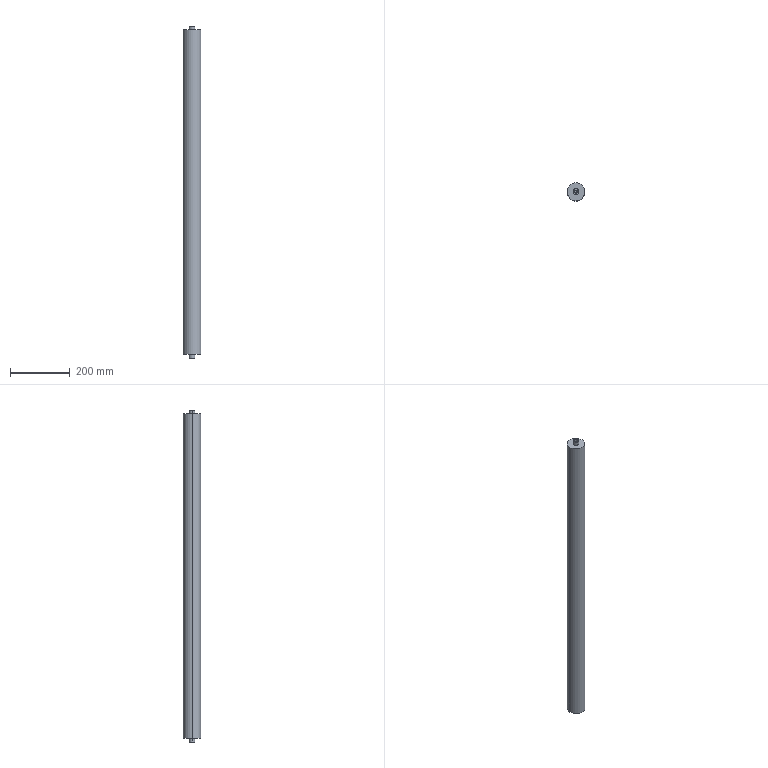Part | SolidWorks | features HoleWzd 2, ICE 2, Extrusion 1 | 1 solid | 18 faces | box 60 x 60 x 1116 mm | volume 3085777 mm3 | cylinder 10 | cone 4 | plane 4 | commonest cylinder face diameters 10.2 x4 20 x4 60 x2
STEP:
#1=CARTESIAN_POINT('',(-5.1,0.,1077.75));
#2=VERTEX_POINT('',#1);
#3=CARTESIAN_POINT('',(5.1,0.,1077.75));
#4=VERTEX_POINT('',#3);
#5=CARTESIAN_POINT('',(0.,0.,1077.75));
#6=DIRECTION('',(0.,0.,1.));
#7=DIRECTION('',(1.,0.,0.));
#8=AXIS2_PLACEMENT_3D('',#5,#6,#7);
#9=CIRCLE('',#8,5.1);
#10=EDGE_CURVE('',#2,#4,#9,.T.);
#11=ORIENTED_EDGE('',*,*,#10,.F.);
#12=CARTESIAN_POINT('',(-5.1,0.,1103.));
#13=VERTEX_POINT('',#12);
#14=CARTESIAN_POINT('',(-5.1,0.,1103.));
#15=DIRECTION('',(0.,0.,1.));
#16=VECTOR('',#15,1000.);
#17=LINE('',#14,#16);
#18=EDGE_CURVE('',#2,#13,#17,.T.);
#19=ORIENTED_EDGE('',*,*,#18,.T.);
#20=CARTESIAN_POINT('',(5.1,0.,1103.));
#21=VERTEX_POINT('',#20);
#22=CARTESIAN_POINT('',(0.,0.,1103.));
#23=DIRECTION('',(0.,0.,1.));
#24=DIRECTION('',(1.,0.,0.));
#25=AXIS2_PLACEMENT_3D('',#22,#23,#24);
#26=CIRCLE('',#25,5.1);
#27=EDGE_CURVE('',#13,#21,#26,.T.);
#28=ORIENTED_EDGE('',*,*,#27,.T.);
#29=CARTESIAN_POINT('',(5.1,0.,1103.));
#30=DIRECTION('',(0.,0.,1.));
#31=VECTOR('',#30,1000.);
#32=LINE('',#29,#31);
#33=EDGE_CURVE('',#4,#21,#32,.T.);
#34=ORIENTED_EDGE('',*,*,#33,.F.);
#35=EDGE_LOOP('',(#11,#19,#28,#34));
#36=FACE_OUTER_BOUND('',#35,.T.);
#37=CARTESIAN_POINT('',(0.,0.,1103.));
#38=DIRECTION('',(0.,0.,1.));
#39=DIRECTION('',(1.,0.,0.));
#40=AXIS2_PLACEMENT_3D('',#37,#38,#39);
#41=CYLINDRICAL_SURFACE('',#40,5.1);
#42=ADVANCED_FACE('',(#36),#41,.F.);
#43=CARTESIAN_POINT('',(0.,0.,1074.686));
#44=VERTEX_POINT('',#43);
#45=CARTESIAN_POINT('',(5.1,0.,1077.75));
#46=DIRECTION('',(0.8572,0.,0.515));
#47=VECTOR('',#46,1000.);
#48=LINE('',#45,#47);
#49=EDGE_CURVE('',#44,#4,#48,.T.);
#50=ORIENTED_EDGE('',*,*,#49,.F.);
#51=CARTESIAN_POINT('',(-5.1,0.,1077.75));
#52=DIRECTION('',(-0.8572,0.,0.515));
#53=VECTOR('',#52,1000.);
#54=LINE('',#51,#53);
#55=EDGE_CURVE('',#44,#2,#54,.T.);
#56=ORIENTED_EDGE('',*,*,#55,.T.);
#57=ORIENTED_EDGE('',*,*,#10,.T.);
#58=EDGE_LOOP('',(#50,#56,#57));
#59=FACE_OUTER_BOUND('',#58,.T.);
#60=CARTESIAN_POINT('',(0.,0.,1077.75));
#61=DIRECTION('',(0.,0.,1.));
#62=DIRECTION('',(1.,0.,0.));
#63=AXIS2_PLACEMENT_3D('',#60,#61,#62);
#64=CONICAL_SURFACE('',#63,5.1,1.03);
#65=ADVANCED_FACE('',(#59),#64,.F.);
#66=CARTESIAN_POINT('',(5.1,0.,12.25));
#67=VERTEX_POINT('',#66);
#68=CARTESIAN_POINT('',(-5.1,0.,12.25));
#69=VERTEX_POINT('',#68);
#70=CARTESIAN_POINT('',(0.,0.,12.25));
#71=DIRECTION('',(0.,0.,-1.));
#72=DIRECTION('',(-1.,0.,0.));
#73=AXIS2_PLACEMENT_3D('',#70,#71,#72);
#74=CIRCLE('',#73,5.1);
#75=EDGE_CURVE('',#67,#69,#74,.T.);
#76=ORIENTED_EDGE('',*,*,#75,.F.);
#77=CARTESIAN_POINT('',(5.1,0.,-13.));
#78=VERTEX_POINT('',#77);
#79=CARTESIAN_POINT('',(5.1,0.,-13.));
#80=DIRECTION('',(0.,0.,-1.));
#81=VECTOR('',#80,1000.);
#82=LINE('',#79,#81);
#83=EDGE_CURVE('',#67,#78,#82,.T.);
#84=ORIENTED_EDGE('',*,*,#83,.T.);
#85=CARTESIAN_POINT('',(-5.1,0.,-13.));
#86=VERTEX_POINT('',#85);
#87=CARTESIAN_POINT('',(0.,0.,-13.));
#88=DIRECTION('',(0.,0.,-1.));
#89=DIRECTION('',(-1.,0.,0.));
#90=AXIS2_PLACEMENT_3D('',#87,#88,#89);
#91=CIRCLE('',#90,5.1);
#92=EDGE_CURVE('',#78,#86,#91,.T.);
#93=ORIENTED_EDGE('',*,*,#92,.T.);
#94=CARTESIAN_POINT('',(-5.1,0.,-13.));
#95=DIRECTION('',(0.,0.,-1.));
#96=VECTOR('',#95,1000.);
#97=LINE('',#94,#96);
#98=EDGE_CURVE('',#69,#86,#97,.T.);
#99=ORIENTED_EDGE('',*,*,#98,.F.);
#100=EDGE_LOOP('',(#76,#84,#93,#99));
#101=FACE_OUTER_BOUND('',#100,.T.);
#102=CARTESIAN_POINT('',(0.,0.,-13.));
#103=DIRECTION('',(0.,0.,-1.));
#104=DIRECTION('',(-1.,0.,0.));
#105=AXIS2_PLACEMENT_3D('',#102,#103,#104);
#106=CYLINDRICAL_SURFACE('',#105,5.1);
#107=ADVANCED_FACE('',(#101),#106,.F.);
#108=CARTESIAN_POINT('',(0.,0.,15.314));
#109=VERTEX_POINT('',#108);
#110=CARTESIAN_POINT('',(-5.1,0.,12.25));
#111=DIRECTION('',(-0.8572,0.,-0.515));
#112=VECTOR('',#111,1000.);
#113=LINE('',#110,#112);
#114=EDGE_CURVE('',#109,#69,#113,.T.);
#115=ORIENTED_EDGE('',*,*,#114,.F.);
#116=CARTESIAN_POINT('',(5.1,0.,12.25));
#117=DIRECTION('',(0.8572,0.,-0.515));
#118=VECTOR('',#117,1000.);
#119=LINE('',#116,#118);
#120=EDGE_CURVE('',#109,#67,#119,.T.);
#121=ORIENTED_EDGE('',*,*,#120,.T.);
#122=ORIENTED_EDGE('',*,*,#75,.T.);
#123=EDGE_LOOP('',(#115,#121,#122));
#124=FACE_OUTER_BOUND('',#123,.T.);
#125=CARTESIAN_POINT('',(0.,0.,12.25));
#126=DIRECTION('',(0.,0.,-1.));
#127=DIRECTION('',(-1.,0.,0.));
#128=AXIS2_PLACEMENT_3D('',#125,#126,#127);
#129=CONICAL_SURFACE('',#128,5.1,1.03);
#130=ADVANCED_FACE('',(#124),#129,.F.);
#131=CARTESIAN_POINT('',(-10.,0.,-13.));
#132=VERTEX_POINT('',#131);
#133=CARTESIAN_POINT('',(10.,0.,-13.));
#134=VERTEX_POINT('',#133);
#135=CARTESIAN_POINT('',(0.,0.,-13.));
#136=DIRECTION('',(0.,0.,-1.));
#137=DIRECTION('',(-1.,0.,0.));
#138=AXIS2_PLACEMENT_3D('',#135,#136,#137);
#139=CIRCLE('',#138,10.);
#140=EDGE_CURVE('',#132,#134,#139,.T.);
#141=ORIENTED_EDGE('',*,*,#140,.F.);
#142=CARTESIAN_POINT('',(-10.,0.,0.));
#143=VERTEX_POINT('',#142);
#144=CARTESIAN_POINT('',(-10.,0.,-13.));
#145=DIRECTION('',(0.,0.,1.));
#146=VECTOR('',#145,1000.);
#147=LINE('',#144,#146);
#148=EDGE_CURVE('',#132,#143,#147,.T.);
#149=ORIENTED_EDGE('',*,*,#148,.T.);
#150=CARTESIAN_POINT('',(10.,0.,0.));
#151=VERTEX_POINT('',#150);
#152=CARTESIAN_POINT('',(0.,0.,0.));
#153=DIRECTION('',(0.,0.,-1.));
#154=DIRECTION('',(-1.,0.,0.));
#155=AXIS2_PLACEMENT_3D('',#152,#153,#154);
#156=CIRCLE('',#155,10.);
#157=EDGE_CURVE('',#143,#151,#156,.T.);
#158=ORIENTED_EDGE('',*,*,#157,.T.);
#159=CARTESIAN_POINT('',(10.,0.,-13.));
#160=DIRECTION('',(0.,0.,1.));
#161=VECTOR('',#160,1000.);
#162=LINE('',#159,#161);
#163=EDGE_CURVE('',#134,#151,#162,.T.);
#164=ORIENTED_EDGE('',*,*,#163,.F.);
#165=EDGE_LOOP('',(#141,#149,#158,#164));
#166=FACE_OUTER_BOUND('',#165,.T.);
#167=CARTESIAN_POINT('',(0.,0.,-13.));
#168=DIRECTION('',(0.,0.,1.));
#169=DIRECTION('',(1.,0.,0.));
#170=AXIS2_PLACEMENT_3D('',#167,#168,#169);
#171=CYLINDRICAL_SURFACE('',#170,10.);
#172=ADVANCED_FACE('',(#166),#171,.T.);
#173=CARTESIAN_POINT('',(10.,0.,1103.));
#174=VERTEX_POINT('',#173);
#175=CARTESIAN_POINT('',(-10.,0.,1103.));
#176=VERTEX_POINT('',#175);
#177=CARTESIAN_POINT('',(0.,0.,1103.));
#178=DIRECTION('',(0.,0.,1.));
#179=DIRECTION('',(1.,0.,0.));
#180=AXIS2_PLACEMENT_3D('',#177,#178,#179);
#181=CIRCLE('',#180,10.);
#182=EDGE_CURVE('',#174,#176,#181,.T.);
#183=ORIENTED_EDGE('',*,*,#182,.F.);
#184=CARTESIAN_POINT('',(10.,0.,1090.));
#185=VERTEX_POINT('',#184);
#186=CARTESIAN_POINT('',(10.,0.,1103.));
#187=DIRECTION('',(0.,0.,-1.));
#188=VECTOR('',#187,1000.);
#189=LINE('',#186,#188);
#190=EDGE_CURVE('',#174,#185,#189,.T.);
#191=ORIENTED_EDGE('',*,*,#190,.T.);
#192=CARTESIAN_POINT('',(-10.,0.,1090.));
#193=VERTEX_POINT('',#192);
#194=CARTESIAN_POINT('',(0.,0.,1090.));
#195=DIRECTION('',(0.,0.,1.));
#196=DIRECTION('',(1.,0.,0.));
#197=AXIS2_PLACEMENT_3D('',#194,#195,#196);
#198=CIRCLE('',#197,10.);
#199=EDGE_CURVE('',#185,#193,#198,.T.);
#200=ORIENTED_EDGE('',*,*,#199,.T.);
#201=CARTESIAN_POINT('',(-10.,0.,1103.));
#202=DIRECTION('',(0.,0.,-1.));
#203=VECTOR('',#202,1000.);
#204=LINE('',#201,#203);
#205=EDGE_CURVE('',#176,#193,#204,.T.);
#206=ORIENTED_EDGE('',*,*,#205,.F.);
#207=EDGE_LOOP('',(#183,#191,#200,#206));
#208=FACE_OUTER_BOUND('',#207,.T.);
#209=CARTESIAN_POINT('',(0.,0.,1103.));
#210=DIRECTION('',(0.,0.,-1.));
#211=DIRECTION('',(-1.,0.,0.));
#212=AXIS2_PLACEMENT_3D('',#209,#210,#211);
#213=CYLINDRICAL_SURFACE('',#212,10.);
#214=ADVANCED_FACE('',(#208),#213,.T.);
#215=CARTESIAN_POINT('',(30.,0.,1090.));
#216=VERTEX_POINT('',#215);
#217=CARTESIAN_POINT('',(-30.,0.,1090.));
#218=VERTEX_POINT('',#217);
#219=CARTESIAN_POINT('',(0.,0.,1090.));
#220=DIRECTION('',(0.,0.,1.));
#221=DIRECTION('',(1.,0.,0.));
#222=AXIS2_PLACEMENT_3D('',#219,#220,#221);
#223=CIRCLE('',#222,30.);
#224=EDGE_CURVE('',#216,#218,#223,.T.);
#225=ORIENTED_EDGE('',*,*,#224,.F.);
#226=CARTESIAN_POINT('',(30.,0.,0.));
#227=VERTEX_POINT('',#226);
#228=CARTESIAN_POINT('',(30.,0.,1090.));
#229=DIRECTION('',(0.,0.,-1.));
#230=VECTOR('',#229,1000.);
#231=LINE('',#228,#230);
#232=EDGE_CURVE('',#216,#227,#231,.T.);
#233=ORIENTED_EDGE('',*,*,#232,.T.);
#234=CARTESIAN_POINT('',(-30.,0.,0.));
#235=VERTEX_POINT('',#234);
#236=CARTESIAN_POINT('',(0.,0.,0.));
#237=DIRECTION('',(0.,0.,1.));
#238=DIRECTION('',(1.,0.,0.));
#239=AXIS2_PLACEMENT_3D('',#236,#237,#238);
#240=CIRCLE('',#239,30.);
#241=EDGE_CURVE('',#227,#235,#240,.T.);
#242=ORIENTED_EDGE('',*,*,#241,.T.);
#243=CARTESIAN_POINT('',(-30.,0.,1090.));
#244=DIRECTION('',(0.,0.,-1.));
#245=VECTOR('',#244,1000.);
#246=LINE('',#243,#245);
#247=EDGE_CURVE('',#218,#235,#246,.T.);
#248=ORIENTED_EDGE('',*,*,#247,.F.);
#249=EDGE_LOOP('',(#225,#233,#242,#248));
#250=FACE_OUTER_BOUND('',#249,.T.);
#251=CARTESIAN_POINT('',(0.,0.,1090.));
#252=DIRECTION('',(0.,0.,-1.));
#253=DIRECTION('',(-1.,0.,0.));
#254=AXIS2_PLACEMENT_3D('',#251,#252,#253);
#255=CYLINDRICAL_SURFACE('',#254,30.);
#256=ADVANCED_FACE('',(#250),#255,.T.);
#257=ORIENTED_EDGE('',*,*,#232,.F.);
#258=CARTESIAN_POINT('',(0.,0.,1090.));
#259=DIRECTION('',(0.,0.,1.));
#260=DIRECTION('',(1.,0.,0.));
#261=AXIS2_PLACEMENT_3D('',#258,#259,#260);
#262=CIRCLE('',#261,30.);
#263=EDGE_CURVE('',#218,#216,#262,.T.);
#264=ORIENTED_EDGE('',*,*,#263,.F.);
#265=ORIENTED_EDGE('',*,*,#247,.T.);
#266=CARTESIAN_POINT('',(0.,0.,0.));
#267=DIRECTION('',(0.,0.,1.));
#268=DIRECTION('',(1.,0.,0.));
#269=AXIS2_PLACEMENT_3D('',#266,#267,#268);
#270=CIRCLE('',#269,30.);
#271=EDGE_CURVE('',#235,#227,#270,.T.);
#272=ORIENTED_EDGE('',*,*,#271,.T.);
#273=EDGE_LOOP('',(#257,#264,#265,#272));
#274=FACE_OUTER_BOUND('',#273,.T.);
#275=CARTESIAN_POINT('',(0.,0.,1090.));
#276=DIRECTION('',(0.,0.,-1.));
#277=DIRECTION('',(-1.,0.,0.));
#278=AXIS2_PLACEMENT_3D('',#275,#276,#277);
#279=CYLINDRICAL_SURFACE('',#278,30.);
#280=ADVANCED_FACE('',(#274),#279,.T.);
#281=CARTESIAN_POINT('',(0.,0.,1090.));
#282=DIRECTION('',(0.,0.,1.));
#283=DIRECTION('',(1.,0.,0.));
#284=AXIS2_PLACEMENT_3D('',#281,#282,#283);
#285=CIRCLE('',#284,10.);
#286=EDGE_CURVE('',#193,#185,#285,.T.);
#287=ORIENTED_EDGE('',*,*,#286,.F.);
#288=ORIENTED_EDGE('',*,*,#199,.F.);
#289=EDGE_LOOP('',(#287,#288));
#290=FACE_BOUND('',#289,.T.);
#291=ORIENTED_EDGE('',*,*,#263,.T.);
#292=ORIENTED_EDGE('',*,*,#224,.T.);
#293=EDGE_LOOP('',(#291,#292));
#294=FACE_OUTER_BOUND('',#293,.T.);
#295=CARTESIAN_POINT('',(0.,0.,1090.));
#296=DIRECTION('',(0.,0.,1.));
#297=DIRECTION('',(1.,0.,0.));
#298=AXIS2_PLACEMENT_3D('',#295,#296,#297);
#299=PLANE('',#298);
#300=ADVANCED_FACE('',(#290,#294),#299,.T.);
#301=CARTESIAN_POINT('',(0.,0.,0.));
#302=DIRECTION('',(0.,0.,-1.));
#303=DIRECTION('',(-1.,0.,0.));
#304=AXIS2_PLACEMENT_3D('',#301,#302,#303);
#305=CIRCLE('',#304,10.);
#306=EDGE_CURVE('',#151,#143,#305,.T.);
#307=ORIENTED_EDGE('',*,*,#306,.F.);
#308=ORIENTED_EDGE('',*,*,#157,.F.);
#309=EDGE_LOOP('',(#307,#308));
#310=FACE_BOUND('',#309,.T.);
#311=ORIENTED_EDGE('',*,*,#271,.F.);
#312=ORIENTED_EDGE('',*,*,#241,.F.);
#313=EDGE_LOOP('',(#311,#312));
#314=FACE_OUTER_BOUND('',#313,.T.);
#315=CARTESIAN_POINT('',(0.,0.,0.));
#316=DIRECTION('',(0.,0.,1.));
#317=DIRECTION('',(1.,0.,0.));
#318=AXIS2_PLACEMENT_3D('',#315,#316,#317);
#319=PLANE('',#318);
#320=ADVANCED_FACE('',(#310,#314),#319,.F.);
#321=ORIENTED_EDGE('',*,*,#190,.F.);
#322=CARTESIAN_POINT('',(0.,0.,1103.));
#323=DIRECTION('',(0.,0.,1.));
#324=DIRECTION('',(1.,0.,0.));
#325=AXIS2_PLACEMENT_3D('',#322,#323,#324);
#326=CIRCLE('',#325,10.);
#327=EDGE_CURVE('',#176,#174,#326,.T.);
#328=ORIENTED_EDGE('',*,*,#327,.F.);
#329=ORIENTED_EDGE('',*,*,#205,.T.);
#330=ORIENTED_EDGE('',*,*,#286,.T.);
#331=EDGE_LOOP('',(#321,#328,#329,#330));
#332=FACE_OUTER_BOUND('',#331,.T.);
#333=CARTESIAN_POINT('',(0.,0.,1103.));
#334=DIRECTION('',(0.,0.,-1.));
#335=DIRECTION('',(-1.,0.,0.));
#336=AXIS2_PLACEMENT_3D('',#333,#334,#335);
#337=CYLINDRICAL_SURFACE('',#336,10.);
#338=ADVANCED_FACE('',(#332),#337,.T.);
#339=CARTESIAN_POINT('',(0.,0.,1103.));
#340=DIRECTION('',(0.,0.,1.));
#341=DIRECTION('',(1.,0.,0.));
#342=AXIS2_PLACEMENT_3D('',#339,#340,#341);
#343=CIRCLE('',#342,5.1);
#344=EDGE_CURVE('',#21,#13,#343,.T.);
#345=ORIENTED_EDGE('',*,*,#344,.F.);
#346=ORIENTED_EDGE('',*,*,#27,.F.);
#347=EDGE_LOOP('',(#345,#346));
#348=FACE_BOUND('',#347,.T.);
#349=ORIENTED_EDGE('',*,*,#327,.T.);
#350=ORIENTED_EDGE('',*,*,#182,.T.);
#351=EDGE_LOOP('',(#349,#350));
#352=FACE_OUTER_BOUND('',#351,.T.);
#353=CARTESIAN_POINT('',(0.,0.,1103.));
#354=DIRECTION('',(0.,0.,1.));
#355=DIRECTION('',(1.,0.,0.));
#356=AXIS2_PLACEMENT_3D('',#353,#354,#355);
#357=PLANE('',#356);
#358=ADVANCED_FACE('',(#348,#352),#357,.T.);
#359=ORIENTED_EDGE('',*,*,#148,.F.);
#360=CARTESIAN_POINT('',(0.,0.,-13.));
#361=DIRECTION('',(0.,0.,-1.));
#362=DIRECTION('',(-1.,0.,0.));
#363=AXIS2_PLACEMENT_3D('',#360,#361,#362);
#364=CIRCLE('',#363,10.);
#365=EDGE_CURVE('',#134,#132,#364,.T.);
#366=ORIENTED_EDGE('',*,*,#365,.F.);
#367=ORIENTED_EDGE('',*,*,#163,.T.);
#368=ORIENTED_EDGE('',*,*,#306,.T.);
#369=EDGE_LOOP('',(#359,#366,#367,#368));
#370=FACE_OUTER_BOUND('',#369,.T.);
#371=CARTESIAN_POINT('',(0.,0.,-13.));
#372=DIRECTION('',(0.,0.,1.));
#373=DIRECTION('',(1.,0.,0.));
#374=AXIS2_PLACEMENT_3D('',#371,#372,#373);
#375=CYLINDRICAL_SURFACE('',#374,10.);
#376=ADVANCED_FACE('',(#370),#375,.T.);
#377=CARTESIAN_POINT('',(0.,0.,-13.));
#378=DIRECTION('',(0.,0.,-1.));
#379=DIRECTION('',(-1.,0.,0.));
#380=AXIS2_PLACEMENT_3D('',#377,#378,#379);
#381=CIRCLE('',#380,5.1);
#382=EDGE_CURVE('',#86,#78,#381,.T.);
#383=ORIENTED_EDGE('',*,*,#382,.F.);
#384=ORIENTED_EDGE('',*,*,#92,.F.);
#385=EDGE_LOOP('',(#383,#384));
#386=FACE_BOUND('',#385,.T.);
#387=ORIENTED_EDGE('',*,*,#365,.T.);
#388=ORIENTED_EDGE('',*,*,#140,.T.);
#389=EDGE_LOOP('',(#387,#388));
#390=FACE_OUTER_BOUND('',#389,.T.);
#391=CARTESIAN_POINT('',(0.,0.,-13.));
#392=DIRECTION('',(0.,0.,-1.));
#393=DIRECTION('',(-1.,0.,0.));
#394=AXIS2_PLACEMENT_3D('',#391,#392,#393);
#395=PLANE('',#394);
#396=ADVANCED_FACE('',(#386,#390),#395,.T.);
#397=ORIENTED_EDGE('',*,*,#120,.F.);
#398=ORIENTED_EDGE('',*,*,#114,.T.);
#399=CARTESIAN_POINT('',(0.,0.,12.25));
#400=DIRECTION('',(0.,0.,-1.));
#401=DIRECTION('',(-1.,0.,0.));
#402=AXIS2_PLACEMENT_3D('',#399,#400,#401);
#403=CIRCLE('',#402,5.1);
#404=EDGE_CURVE('',#69,#67,#403,.T.);
#405=ORIENTED_EDGE('',*,*,#404,.T.);
#406=EDGE_LOOP('',(#397,#398,#405));
#407=FACE_OUTER_BOUND('',#406,.T.);
#408=CARTESIAN_POINT('',(0.,0.,12.25));
#409=DIRECTION('',(0.,0.,-1.));
#410=DIRECTION('',(-1.,0.,0.));
#411=AXIS2_PLACEMENT_3D('',#408,#409,#410);
#412=CONICAL_SURFACE('',#411,5.1,1.03);
#413=ADVANCED_FACE('',(#407),#412,.F.);
#414=ORIENTED_EDGE('',*,*,#83,.F.);
#415=ORIENTED_EDGE('',*,*,#404,.F.);
#416=ORIENTED_EDGE('',*,*,#98,.T.);
#417=ORIENTED_EDGE('',*,*,#382,.T.);
#418=EDGE_LOOP('',(#414,#415,#416,#417));
#419=FACE_OUTER_BOUND('',#418,.T.);
#420=CARTESIAN_POINT('',(0.,0.,-13.));
#421=DIRECTION('',(0.,0.,-1.));
#422=DIRECTION('',(-1.,0.,0.));
#423=AXIS2_PLACEMENT_3D('',#420,#421,#422);
#424=CYLINDRICAL_SURFACE('',#423,5.1);
#425=ADVANCED_FACE('',(#419),#424,.F.);
#426=ORIENTED_EDGE('',*,*,#55,.F.);
#427=ORIENTED_EDGE('',*,*,#49,.T.);
#428=CARTESIAN_POINT('',(0.,0.,1077.75));
#429=DIRECTION('',(0.,0.,1.));
#430=DIRECTION('',(1.,0.,0.));
#431=AXIS2_PLACEMENT_3D('',#428,#429,#430);
#432=CIRCLE('',#431,5.1);
#433=EDGE_CURVE('',#4,#2,#432,.T.);
#434=ORIENTED_EDGE('',*,*,#433,.T.);
#435=EDGE_LOOP('',(#426,#427,#434));
#436=FACE_OUTER_BOUND('',#435,.T.);
#437=CARTESIAN_POINT('',(0.,0.,1077.75));
#438=DIRECTION('',(0.,0.,1.));
#439=DIRECTION('',(1.,0.,0.));
#440=AXIS2_PLACEMENT_3D('',#437,#438,#439);
#441=CONICAL_SURFACE('',#440,5.1,1.03);
#442=ADVANCED_FACE('',(#436),#441,.F.);
#443=ORIENTED_EDGE('',*,*,#18,.F.);
#444=ORIENTED_EDGE('',*,*,#433,.F.);
#445=ORIENTED_EDGE('',*,*,#33,.T.);
#446=ORIENTED_EDGE('',*,*,#344,.T.);
#447=EDGE_LOOP('',(#443,#444,#445,#446));
#448=FACE_OUTER_BOUND('',#447,.T.);
#449=CARTESIAN_POINT('',(0.,0.,1103.));
#450=DIRECTION('',(0.,0.,1.));
#451=DIRECTION('',(1.,0.,0.));
#452=AXIS2_PLACEMENT_3D('',#449,#450,#451);
#453=CYLINDRICAL_SURFACE('',#452,5.1);
#454=ADVANCED_FACE('',(#448),#453,.F.);
#455=CLOSED_SHELL('',(#42,#65,#107,#130,#172,#214,#256,#280,#300,#320,#338,#358,#376,#396,#413,#425,#442,#454));
#456=MANIFOLD_SOLID_BREP('',#455);
#457=CARTESIAN_POINT('',(0.,0.,0.));
#458=DIRECTION('',(0.,0.,1.));
#459=DIRECTION('',(1.,0.,0.));
#460=AXIS2_PLACEMENT_3D('',#457,#458,#459);
#461=(LENGTH_UNIT()NAMED_UNIT(*)SI_UNIT(.MILLI.,.METRE.));
#462=UNCERTAINTY_MEASURE_WITH_UNIT(LENGTH_MEASURE(0.00001),#461,'','');
#463=(NAMED_UNIT(*)PLANE_ANGLE_UNIT()SI_UNIT($,.RADIAN.));
#464=(NAMED_UNIT(*)SI_UNIT($,.STERADIAN.)SOLID_ANGLE_UNIT());
#465=(GEOMETRIC_REPRESENTATION_CONTEXT(3)GLOBAL_UNCERTAINTY_ASSIGNED_CONTEXT((#462))GLOBAL_UNIT_ASSIGNED_CONTEXT((#461,#463,#464))REPRESENTATION_CONTEXT('',''));
#466=ADVANCED_BREP_SHAPE_REPRESENTATION('',(#456,#460),#465);